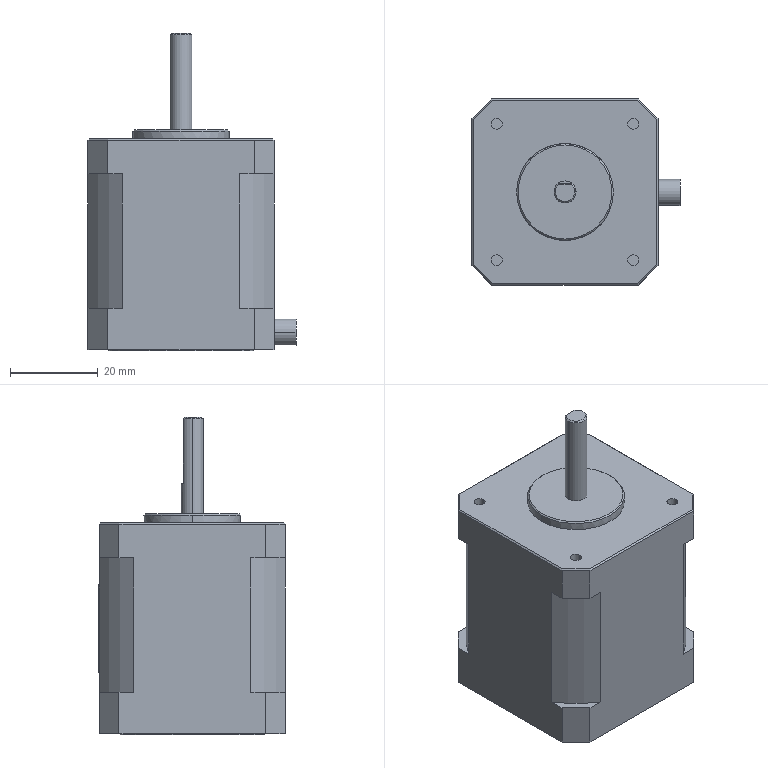Part | NX | features BREP 1 | 1 solid | 1845 faces | box 47.3 x 42.4 x 72.2 mm | volume 83104 mm3 | plane 1223 | spline 393 | cylinder 160 | cone 49 | torus 16 | sphere 4 | commonest cylinder face diameters 0.073 x9 2.5 x8 3 x8 3.5 x8 5.6 x8 6.2 x8